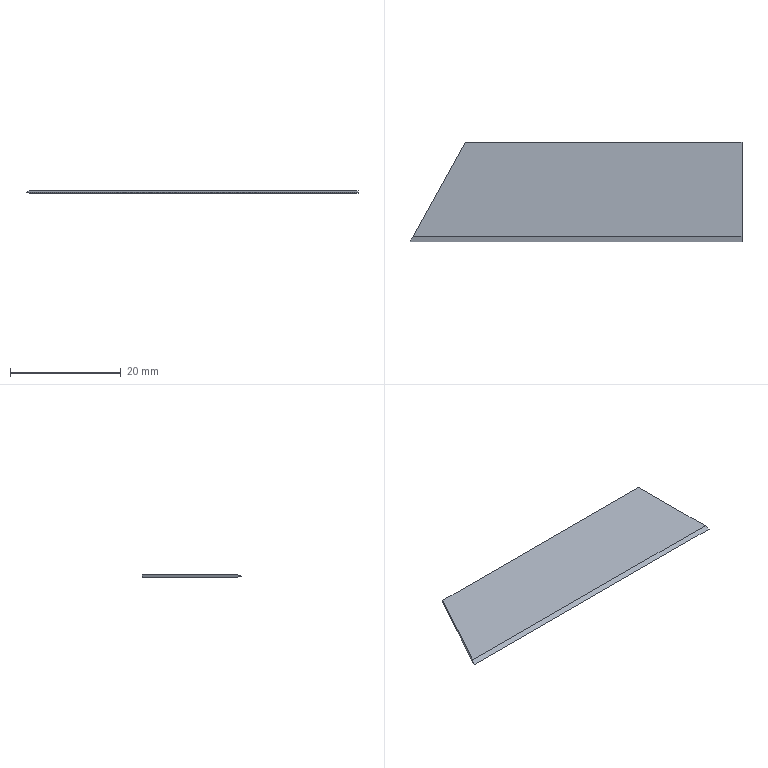Part | STEP file | Mount electronic clip blade | 1 solid | 7 faces | box 60 x 18 x 0.5 mm | volume 480.046 mm3 | plane 7
STEP:
#1=CARTESIAN_POINT('',(0.,0.,0.));
#2=DIRECTION('',(0.,0.,1.));
#3=DIRECTION('',(1.,0.,0.));
#4=AXIS2_PLACEMENT_3D('',#1,#2,#3);
#5=CARTESIAN_POINT('',(30.,-8.,0.5));
#6=VERTEX_POINT('',#5);
#7=CARTESIAN_POINT('',(30.,9.,0.5));
#8=VERTEX_POINT('',#7);
#9=CARTESIAN_POINT('',(30.,-9.,0.5));
#10=DIRECTION('',(0.,1.,0.));
#11=VECTOR('',#10,1.);
#12=LINE('',#9,#11);
#13=CARTESIAN_POINT('',(30.,-9.,0.5));
#14=DIRECTION('',(-1.,0.,0.));
#15=DIRECTION('',(0.,0.,1.));
#16=AXIS2_PLACEMENT_3D('',#13,#14,#15);
#17=PLANE('',#16);
#18=CARTESIAN_POINT('',(0.,0.));
#19=DIRECTION('',(0.,1.));
#20=VECTOR('',#19,1.);
#21=LINE('',#18,#20);
#22=(GEOMETRIC_REPRESENTATION_CONTEXT(2)PARAMETRIC_REPRESENTATION_CONTEXT()REPRESENTATION_CONTEXT('',''));
#23=DEFINITIONAL_REPRESENTATION('',(#21),#22);
#24=PCURVE('',#17,#23);
#25=CARTESIAN_POINT('',(0.,0.,0.5));
#26=DIRECTION('',(0.,0.,-1.));
#27=DIRECTION('',(-1.,0.,0.));
#28=AXIS2_PLACEMENT_3D('',#25,#26,#27);
#29=PLANE('',#28);
#30=CARTESIAN_POINT('',(-30.,-9.));
#31=DIRECTION('',(0.,1.));
#32=VECTOR('',#31,1.);
#33=LINE('',#30,#32);
#34=(GEOMETRIC_REPRESENTATION_CONTEXT(2)PARAMETRIC_REPRESENTATION_CONTEXT()REPRESENTATION_CONTEXT('',''));
#35=DEFINITIONAL_REPRESENTATION('',(#33),#34);
#36=PCURVE('',#29,#35);
#37=SURFACE_CURVE('',#12,(#24,#36),.PCURVE_S1.);
#38=EDGE_CURVE('',#6,#8,#37,.T.);
#39=ORIENTED_EDGE('',*,*,#38,.F.);
#40=CARTESIAN_POINT('',(30.,-9.,0.25));
#41=VERTEX_POINT('',#40);
#42=CARTESIAN_POINT('',(30.,-8.,0.5));
#43=DIRECTION('',(0.,-0.9701,-0.2425));
#44=VECTOR('',#43,1.);
#45=LINE('',#42,#44);
#46=CARTESIAN_POINT('',(0.,1.));
#47=DIRECTION('',(-0.2425,-0.9701));
#48=VECTOR('',#47,1.);
#49=LINE('',#46,#48);
#50=(GEOMETRIC_REPRESENTATION_CONTEXT(2)PARAMETRIC_REPRESENTATION_CONTEXT()REPRESENTATION_CONTEXT('',''));
#51=DEFINITIONAL_REPRESENTATION('',(#49),#50);
#52=PCURVE('',#17,#51);
#53=CARTESIAN_POINT('',(0.,-8.,0.5));
#54=DIRECTION('',(0.,0.2425,-0.9701));
#55=DIRECTION('',(1.,0.,0.));
#56=AXIS2_PLACEMENT_3D('',#53,#54,#55);
#57=PLANE('',#56);
#58=CARTESIAN_POINT('',(30.,0.));
#59=DIRECTION('',(0.,1.));
#60=VECTOR('',#59,1.);
#61=LINE('',#58,#60);
#62=(GEOMETRIC_REPRESENTATION_CONTEXT(2)PARAMETRIC_REPRESENTATION_CONTEXT()REPRESENTATION_CONTEXT('',''));
#63=DEFINITIONAL_REPRESENTATION('',(#61),#62);
#64=PCURVE('',#57,#63);
#65=SURFACE_CURVE('',#45,(#52,#64),.PCURVE_S1.);
#66=EDGE_CURVE('',#6,#41,#65,.T.);
#67=ORIENTED_EDGE('',*,*,#66,.T.);
#68=CARTESIAN_POINT('',(30.,-8.,0.));
#69=VERTEX_POINT('',#68);
#70=CARTESIAN_POINT('',(30.,-9.,0.25));
#71=DIRECTION('',(0.,0.9701,-0.2425));
#72=VECTOR('',#71,1.);
#73=LINE('',#70,#72);
#74=CARTESIAN_POINT('',(-0.25,0.));
#75=DIRECTION('',(-0.2425,0.9701));
#76=VECTOR('',#75,1.);
#77=LINE('',#74,#76);
#78=(GEOMETRIC_REPRESENTATION_CONTEXT(2)PARAMETRIC_REPRESENTATION_CONTEXT()REPRESENTATION_CONTEXT('',''));
#79=DEFINITIONAL_REPRESENTATION('',(#77),#78);
#80=PCURVE('',#17,#79);
#81=CARTESIAN_POINT('',(-30.,-9.,0.25));
#82=DIRECTION('',(0.,-0.2425,-0.9701));
#83=DIRECTION('',(-1.,0.,0.));
#84=AXIS2_PLACEMENT_3D('',#81,#82,#83);
#85=PLANE('',#84);
#86=CARTESIAN_POINT('',(-60.,0.));
#87=DIRECTION('',(0.,1.));
#88=VECTOR('',#87,1.);
#89=LINE('',#86,#88);
#90=(GEOMETRIC_REPRESENTATION_CONTEXT(2)PARAMETRIC_REPRESENTATION_CONTEXT()REPRESENTATION_CONTEXT('',''));
#91=DEFINITIONAL_REPRESENTATION('',(#89),#90);
#92=PCURVE('',#85,#91);
#93=SURFACE_CURVE('',#73,(#80,#92),.PCURVE_S1.);
#94=EDGE_CURVE('',#41,#69,#93,.T.);
#95=ORIENTED_EDGE('',*,*,#94,.T.);
#96=CARTESIAN_POINT('',(30.,9.,0.));
#97=VERTEX_POINT('',#96);
#98=CARTESIAN_POINT('',(30.,-9.,0.));
#99=DIRECTION('',(0.,1.,0.));
#100=VECTOR('',#99,1.);
#101=LINE('',#98,#100);
#102=CARTESIAN_POINT('',(-0.5,0.));
#103=DIRECTION('',(0.,1.));
#104=VECTOR('',#103,1.);
#105=LINE('',#102,#104);
#106=(GEOMETRIC_REPRESENTATION_CONTEXT(2)PARAMETRIC_REPRESENTATION_CONTEXT()REPRESENTATION_CONTEXT('',''));
#107=DEFINITIONAL_REPRESENTATION('',(#105),#106);
#108=PCURVE('',#17,#107);
#109=CARTESIAN_POINT('',(0.,0.,0.));
#110=DIRECTION('',(0.,0.,-1.));
#111=DIRECTION('',(-1.,0.,0.));
#112=AXIS2_PLACEMENT_3D('',#109,#110,#111);
#113=PLANE('',#112);
#114=CARTESIAN_POINT('',(-30.,-9.));
#115=DIRECTION('',(0.,1.));
#116=VECTOR('',#115,1.);
#117=LINE('',#114,#116);
#118=(GEOMETRIC_REPRESENTATION_CONTEXT(2)PARAMETRIC_REPRESENTATION_CONTEXT()REPRESENTATION_CONTEXT('',''));
#119=DEFINITIONAL_REPRESENTATION('',(#117),#118);
#120=PCURVE('',#113,#119);
#121=SURFACE_CURVE('',#101,(#108,#120),.PCURVE_S1.);
#122=EDGE_CURVE('',#69,#97,#121,.T.);
#123=ORIENTED_EDGE('',*,*,#122,.T.);
#124=CARTESIAN_POINT('',(30.,9.,0.5));
#125=DIRECTION('',(0.,0.,-1.));
#126=VECTOR('',#125,1.);
#127=LINE('',#124,#126);
#128=CARTESIAN_POINT('',(0.,18.));
#129=DIRECTION('',(-1.,0.));
#130=VECTOR('',#129,1.);
#131=LINE('',#128,#130);
#132=(GEOMETRIC_REPRESENTATION_CONTEXT(2)PARAMETRIC_REPRESENTATION_CONTEXT()REPRESENTATION_CONTEXT('',''));
#133=DEFINITIONAL_REPRESENTATION('',(#131),#132);
#134=PCURVE('',#17,#133);
#135=CARTESIAN_POINT('',(-30.,9.,0.5));
#136=DIRECTION('',(0.,-1.,0.));
#137=DIRECTION('',(0.,0.,-1.));
#138=AXIS2_PLACEMENT_3D('',#135,#136,#137);
#139=PLANE('',#138);
#140=CARTESIAN_POINT('',(0.,60.));
#141=DIRECTION('',(1.,0.));
#142=VECTOR('',#141,1.);
#143=LINE('',#140,#142);
#144=(GEOMETRIC_REPRESENTATION_CONTEXT(2)PARAMETRIC_REPRESENTATION_CONTEXT()REPRESENTATION_CONTEXT('',''));
#145=DEFINITIONAL_REPRESENTATION('',(#143),#144);
#146=PCURVE('',#139,#145);
#147=SURFACE_CURVE('',#127,(#134,#146),.PCURVE_S1.);
#148=EDGE_CURVE('',#8,#97,#147,.T.);
#149=ORIENTED_EDGE('',*,*,#148,.F.);
#150=EDGE_LOOP('',(#39,#67,#95,#123,#149));
#151=FACE_BOUND('',#150,.T.);
#152=ADVANCED_FACE('',(#151),#17,.F.);
#153=CARTESIAN_POINT('',(-20.,9.,0.));
#154=VERTEX_POINT('',#153);
#155=CARTESIAN_POINT('',(-30.,9.,0.));
#156=DIRECTION('',(-1.,0.,0.));
#157=VECTOR('',#156,1.);
#158=LINE('',#155,#157);
#159=CARTESIAN_POINT('',(0.5,0.));
#160=DIRECTION('',(0.,-1.));
#161=VECTOR('',#160,1.);
#162=LINE('',#159,#161);
#163=(GEOMETRIC_REPRESENTATION_CONTEXT(2)PARAMETRIC_REPRESENTATION_CONTEXT()REPRESENTATION_CONTEXT('',''));
#164=DEFINITIONAL_REPRESENTATION('',(#162),#163);
#165=PCURVE('',#139,#164);
#166=CARTESIAN_POINT('',(30.,9.));
#167=DIRECTION('',(1.,0.));
#168=VECTOR('',#167,1.);
#169=LINE('',#166,#168);
#170=(GEOMETRIC_REPRESENTATION_CONTEXT(2)PARAMETRIC_REPRESENTATION_CONTEXT()REPRESENTATION_CONTEXT('',''));
#171=DEFINITIONAL_REPRESENTATION('',(#169),#170);
#172=PCURVE('',#113,#171);
#173=SURFACE_CURVE('',#158,(#165,#172),.PCURVE_S1.);
#174=EDGE_CURVE('',#97,#154,#173,.T.);
#175=ORIENTED_EDGE('',*,*,#174,.T.);
#176=CARTESIAN_POINT('',(-20.,9.,0.5));
#177=VERTEX_POINT('',#176);
#178=CARTESIAN_POINT('',(-20.,9.,-1.));
#179=DIRECTION('',(0.,0.,1.));
#180=VECTOR('',#179,1.);
#181=LINE('',#178,#180);
#182=CARTESIAN_POINT('',(1.5,10.));
#183=DIRECTION('',(-1.,0.));
#184=VECTOR('',#183,1.);
#185=LINE('',#182,#184);
#186=(GEOMETRIC_REPRESENTATION_CONTEXT(2)PARAMETRIC_REPRESENTATION_CONTEXT()REPRESENTATION_CONTEXT('',''));
#187=DEFINITIONAL_REPRESENTATION('',(#185),#186);
#188=PCURVE('',#139,#187);
#189=CARTESIAN_POINT('',(-30.,-9.,-1.));
#190=DIRECTION('',(0.8742,-0.4856,0.));
#191=DIRECTION('',(0.4856,0.8742,0.));
#192=AXIS2_PLACEMENT_3D('',#189,#190,#191);
#193=PLANE('',#192);
#194=CARTESIAN_POINT('',(20.591,0.));
#195=DIRECTION('',(0.,1.));
#196=VECTOR('',#195,1.);
#197=LINE('',#194,#196);
#198=(GEOMETRIC_REPRESENTATION_CONTEXT(2)PARAMETRIC_REPRESENTATION_CONTEXT()REPRESENTATION_CONTEXT('',''));
#199=DEFINITIONAL_REPRESENTATION('',(#197),#198);
#200=PCURVE('',#193,#199);
#201=SURFACE_CURVE('',#181,(#188,#200),.PCURVE_S1.);
#202=EDGE_CURVE('',#154,#177,#201,.T.);
#203=ORIENTED_EDGE('',*,*,#202,.T.);
#204=CARTESIAN_POINT('',(-30.,9.,0.5));
#205=DIRECTION('',(-1.,0.,0.));
#206=VECTOR('',#205,1.);
#207=LINE('',#204,#206);
#208=CARTESIAN_POINT('',(0.,0.));
#209=DIRECTION('',(0.,-1.));
#210=VECTOR('',#209,1.);
#211=LINE('',#208,#210);
#212=(GEOMETRIC_REPRESENTATION_CONTEXT(2)PARAMETRIC_REPRESENTATION_CONTEXT()REPRESENTATION_CONTEXT('',''));
#213=DEFINITIONAL_REPRESENTATION('',(#211),#212);
#214=PCURVE('',#139,#213);
#215=CARTESIAN_POINT('',(30.,9.));
#216=DIRECTION('',(1.,0.));
#217=VECTOR('',#216,1.);
#218=LINE('',#215,#217);
#219=(GEOMETRIC_REPRESENTATION_CONTEXT(2)PARAMETRIC_REPRESENTATION_CONTEXT()REPRESENTATION_CONTEXT('',''));
#220=DEFINITIONAL_REPRESENTATION('',(#218),#219);
#221=PCURVE('',#29,#220);
#222=SURFACE_CURVE('',#207,(#214,#221),.PCURVE_S1.);
#223=EDGE_CURVE('',#8,#177,#222,.T.);
#224=ORIENTED_EDGE('',*,*,#223,.F.);
#225=ORIENTED_EDGE('',*,*,#148,.T.);
#226=EDGE_LOOP('',(#175,#203,#224,#225));
#227=FACE_BOUND('',#226,.T.);
#228=ADVANCED_FACE('',(#227),#139,.F.);
#229=CARTESIAN_POINT('',(-29.444,-8.,0.5));
#230=VERTEX_POINT('',#229);
#231=CARTESIAN_POINT('',(-30.,-9.,0.5));
#232=DIRECTION('',(0.4856,0.8742,0.));
#233=VECTOR('',#232,1.);
#234=LINE('',#231,#233);
#235=CARTESIAN_POINT('',(30.,-9.));
#236=DIRECTION('',(-0.4856,0.8742));
#237=VECTOR('',#236,1.);
#238=LINE('',#235,#237);
#239=(GEOMETRIC_REPRESENTATION_CONTEXT(2)PARAMETRIC_REPRESENTATION_CONTEXT()REPRESENTATION_CONTEXT('',''));
#240=DEFINITIONAL_REPRESENTATION('',(#238),#239);
#241=PCURVE('',#29,#240);
#242=CARTESIAN_POINT('',(0.,1.5));
#243=DIRECTION('',(1.,0.));
#244=VECTOR('',#243,1.);
#245=LINE('',#242,#244);
#246=(GEOMETRIC_REPRESENTATION_CONTEXT(2)PARAMETRIC_REPRESENTATION_CONTEXT()REPRESENTATION_CONTEXT('',''));
#247=DEFINITIONAL_REPRESENTATION('',(#245),#246);
#248=PCURVE('',#193,#247);
#249=SURFACE_CURVE('',#234,(#241,#248),.PCURVE_S1.);
#250=EDGE_CURVE('',#230,#177,#249,.T.);
#251=ORIENTED_EDGE('',*,*,#250,.F.);
#252=CARTESIAN_POINT('',(0.,-8.,0.5));
#253=DIRECTION('',(1.,0.,0.));
#254=VECTOR('',#253,1.);
#255=LINE('',#252,#254);
#256=CARTESIAN_POINT('',(0.,-8.));
#257=DIRECTION('',(-1.,0.));
#258=VECTOR('',#257,1.);
#259=LINE('',#256,#258);
#260=(GEOMETRIC_REPRESENTATION_CONTEXT(2)PARAMETRIC_REPRESENTATION_CONTEXT()REPRESENTATION_CONTEXT('',''));
#261=DEFINITIONAL_REPRESENTATION('',(#259),#260);
#262=PCURVE('',#29,#261);
#263=CARTESIAN_POINT('',(0.,0.));
#264=DIRECTION('',(1.,0.));
#265=VECTOR('',#264,1.);
#266=LINE('',#263,#265);
#267=(GEOMETRIC_REPRESENTATION_CONTEXT(2)PARAMETRIC_REPRESENTATION_CONTEXT()REPRESENTATION_CONTEXT('',''));
#268=DEFINITIONAL_REPRESENTATION('',(#266),#267);
#269=PCURVE('',#57,#268);
#270=SURFACE_CURVE('',#255,(#262,#269),.PCURVE_S1.);
#271=EDGE_CURVE('',#230,#6,#270,.T.);
#272=ORIENTED_EDGE('',*,*,#271,.T.);
#273=ORIENTED_EDGE('',*,*,#38,.T.);
#274=ORIENTED_EDGE('',*,*,#223,.T.);
#275=EDGE_LOOP('',(#251,#272,#273,#274));
#276=FACE_BOUND('',#275,.T.);
#277=ADVANCED_FACE('',(#276),#29,.F.);
#278=ORIENTED_EDGE('',*,*,#122,.F.);
#279=CARTESIAN_POINT('',(-29.444,-8.,0.));
#280=VERTEX_POINT('',#279);
#281=CARTESIAN_POINT('',(-30.,-8.,0.));
#282=DIRECTION('',(-1.,0.,0.));
#283=VECTOR('',#282,1.);
#284=LINE('',#281,#283);
#285=CARTESIAN_POINT('',(30.,-8.));
#286=DIRECTION('',(1.,0.));
#287=VECTOR('',#286,1.);
#288=LINE('',#285,#287);
#289=(GEOMETRIC_REPRESENTATION_CONTEXT(2)PARAMETRIC_REPRESENTATION_CONTEXT()REPRESENTATION_CONTEXT('',''));
#290=DEFINITIONAL_REPRESENTATION('',(#288),#289);
#291=PCURVE('',#113,#290);
#292=CARTESIAN_POINT('',(0.,1.031));
#293=DIRECTION('',(1.,0.));
#294=VECTOR('',#293,1.);
#295=LINE('',#292,#294);
#296=(GEOMETRIC_REPRESENTATION_CONTEXT(2)PARAMETRIC_REPRESENTATION_CONTEXT()REPRESENTATION_CONTEXT('',''));
#297=DEFINITIONAL_REPRESENTATION('',(#295),#296);
#298=PCURVE('',#85,#297);
#299=SURFACE_CURVE('',#284,(#291,#298),.PCURVE_S1.);
#300=EDGE_CURVE('',#69,#280,#299,.T.);
#301=ORIENTED_EDGE('',*,*,#300,.T.);
#302=CARTESIAN_POINT('',(-19.104,10.613,0.));
#303=DIRECTION('',(-0.4856,-0.8742,0.));
#304=VECTOR('',#303,1.);
#305=LINE('',#302,#304);
#306=CARTESIAN_POINT('',(19.104,10.613));
#307=DIRECTION('',(0.4856,-0.8742));
#308=VECTOR('',#307,1.);
#309=LINE('',#306,#308);
#310=(GEOMETRIC_REPRESENTATION_CONTEXT(2)PARAMETRIC_REPRESENTATION_CONTEXT()REPRESENTATION_CONTEXT('',''));
#311=DEFINITIONAL_REPRESENTATION('',(#309),#310);
#312=PCURVE('',#113,#311);
#313=CARTESIAN_POINT('',(22.437,1.));
#314=DIRECTION('',(-1.,0.));
#315=VECTOR('',#314,1.);
#316=LINE('',#313,#315);
#317=(GEOMETRIC_REPRESENTATION_CONTEXT(2)PARAMETRIC_REPRESENTATION_CONTEXT()REPRESENTATION_CONTEXT('',''));
#318=DEFINITIONAL_REPRESENTATION('',(#316),#317);
#319=PCURVE('',#193,#318);
#320=SURFACE_CURVE('',#305,(#312,#319),.PCURVE_S1.);
#321=EDGE_CURVE('',#154,#280,#320,.T.);
#322=ORIENTED_EDGE('',*,*,#321,.F.);
#323=ORIENTED_EDGE('',*,*,#174,.F.);
#324=EDGE_LOOP('',(#278,#301,#322,#323));
#325=FACE_BOUND('',#324,.T.);
#326=ADVANCED_FACE('',(#325),#113,.T.);
#327=CARTESIAN_POINT('',(-30.,-9.,0.25));
#328=VERTEX_POINT('',#327);
#329=CARTESIAN_POINT('',(-30.,-9.,0.25));
#330=DIRECTION('',(-0.4744,-0.854,0.2135));
#331=VECTOR('',#330,1.);
#332=LINE('',#329,#331);
#333=CARTESIAN_POINT('',(0.,1.25));
#334=DIRECTION('',(-0.9769,0.2135));
#335=VECTOR('',#334,1.);
#336=LINE('',#333,#335);
#337=(GEOMETRIC_REPRESENTATION_CONTEXT(2)PARAMETRIC_REPRESENTATION_CONTEXT()REPRESENTATION_CONTEXT('',''));
#338=DEFINITIONAL_REPRESENTATION('',(#336),#337);
#339=PCURVE('',#193,#338);
#340=CARTESIAN_POINT('',(0.,0.));
#341=DIRECTION('',(0.4744,-0.8803));
#342=VECTOR('',#341,1.);
#343=LINE('',#340,#342);
#344=(GEOMETRIC_REPRESENTATION_CONTEXT(2)PARAMETRIC_REPRESENTATION_CONTEXT()REPRESENTATION_CONTEXT('',''));
#345=DEFINITIONAL_REPRESENTATION('',(#343),#344);
#346=PCURVE('',#85,#345);
#347=SURFACE_CURVE('',#332,(#339,#346),.PCURVE_S1.);
#348=EDGE_CURVE('',#280,#328,#347,.T.);
#349=ORIENTED_EDGE('',*,*,#348,.T.);
#350=CARTESIAN_POINT('',(-22.817,3.93,3.483));
#351=DIRECTION('',(0.4744,0.854,0.2135));
#352=VECTOR('',#351,1.);
#353=LINE('',#350,#352);
#354=CARTESIAN_POINT('',(14.792,4.483));
#355=DIRECTION('',(0.9769,0.2135));
#356=VECTOR('',#355,1.);
#357=LINE('',#354,#356);
#358=(GEOMETRIC_REPRESENTATION_CONTEXT(2)PARAMETRIC_REPRESENTATION_CONTEXT()REPRESENTATION_CONTEXT('',''));
#359=DEFINITIONAL_REPRESENTATION('',(#357),#358);
#360=PCURVE('',#193,#359);
#361=CARTESIAN_POINT('',(-22.817,-12.297));
#362=DIRECTION('',(0.4744,-0.8803));
#363=VECTOR('',#362,1.);
#364=LINE('',#361,#363);
#365=(GEOMETRIC_REPRESENTATION_CONTEXT(2)PARAMETRIC_REPRESENTATION_CONTEXT()REPRESENTATION_CONTEXT('',''));
#366=DEFINITIONAL_REPRESENTATION('',(#364),#365);
#367=PCURVE('',#57,#366);
#368=SURFACE_CURVE('',#353,(#360,#367),.PCURVE_S1.);
#369=EDGE_CURVE('',#328,#230,#368,.T.);
#370=ORIENTED_EDGE('',*,*,#369,.T.);
#371=ORIENTED_EDGE('',*,*,#250,.T.);
#372=ORIENTED_EDGE('',*,*,#202,.F.);
#373=ORIENTED_EDGE('',*,*,#321,.T.);
#374=EDGE_LOOP('',(#349,#370,#371,#372,#373));
#375=FACE_BOUND('',#374,.T.);
#376=ADVANCED_FACE('',(#375),#193,.F.);
#377=ORIENTED_EDGE('',*,*,#348,.F.);
#378=ORIENTED_EDGE('',*,*,#300,.F.);
#379=ORIENTED_EDGE('',*,*,#94,.F.);
#380=CARTESIAN_POINT('',(30.,-9.,0.25));
#381=DIRECTION('',(1.,0.,0.));
#382=VECTOR('',#381,1.);
#383=LINE('',#380,#382);
#384=CARTESIAN_POINT('',(-60.,0.));
#385=DIRECTION('',(-1.,0.));
#386=VECTOR('',#385,1.);
#387=LINE('',#384,#386);
#388=(GEOMETRIC_REPRESENTATION_CONTEXT(2)PARAMETRIC_REPRESENTATION_CONTEXT()REPRESENTATION_CONTEXT('',''));
#389=DEFINITIONAL_REPRESENTATION('',(#387),#388);
#390=PCURVE('',#85,#389);
#391=CARTESIAN_POINT('',(30.,1.031));
#392=DIRECTION('',(1.,0.));
#393=VECTOR('',#392,1.);
#394=LINE('',#391,#393);
#395=(GEOMETRIC_REPRESENTATION_CONTEXT(2)PARAMETRIC_REPRESENTATION_CONTEXT()REPRESENTATION_CONTEXT('',''));
#396=DEFINITIONAL_REPRESENTATION('',(#394),#395);
#397=PCURVE('',#57,#396);
#398=SURFACE_CURVE('',#383,(#390,#397),.PCURVE_S1.);
#399=EDGE_CURVE('',#328,#41,#398,.T.);
#400=ORIENTED_EDGE('',*,*,#399,.F.);
#401=EDGE_LOOP('',(#377,#378,#379,#400));
#402=FACE_BOUND('',#401,.T.);
#403=ADVANCED_FACE('',(#402),#85,.T.);
#404=ORIENTED_EDGE('',*,*,#369,.F.);
#405=ORIENTED_EDGE('',*,*,#399,.T.);
#406=ORIENTED_EDGE('',*,*,#66,.F.);
#407=ORIENTED_EDGE('',*,*,#271,.F.);
#408=EDGE_LOOP('',(#404,#405,#406,#407));
#409=FACE_BOUND('',#408,.T.);
#410=ADVANCED_FACE('',(#409),#57,.F.);
#411=CLOSED_SHELL('',(#152,#228,#277,#326,#376,#403,#410));
#412=MANIFOLD_SOLID_BREP('',#411);
#413=(LENGTH_UNIT()NAMED_UNIT(*)SI_UNIT(.MILLI.,.METRE.));
#414=UNCERTAINTY_MEASURE_WITH_UNIT(LENGTH_MEASURE(0.0000001),#413,'','');
#415=(NAMED_UNIT(*)PLANE_ANGLE_UNIT()SI_UNIT($,.RADIAN.));
#416=(NAMED_UNIT(*)SI_UNIT($,.STERADIAN.)SOLID_ANGLE_UNIT());
#417=(GEOMETRIC_REPRESENTATION_CONTEXT(3)GLOBAL_UNCERTAINTY_ASSIGNED_CONTEXT((#414))GLOBAL_UNIT_ASSIGNED_CONTEXT((#413,#415,#416))REPRESENTATION_CONTEXT('',''));
#418=ADVANCED_BREP_SHAPE_REPRESENTATION('',(#4,#412),#417);